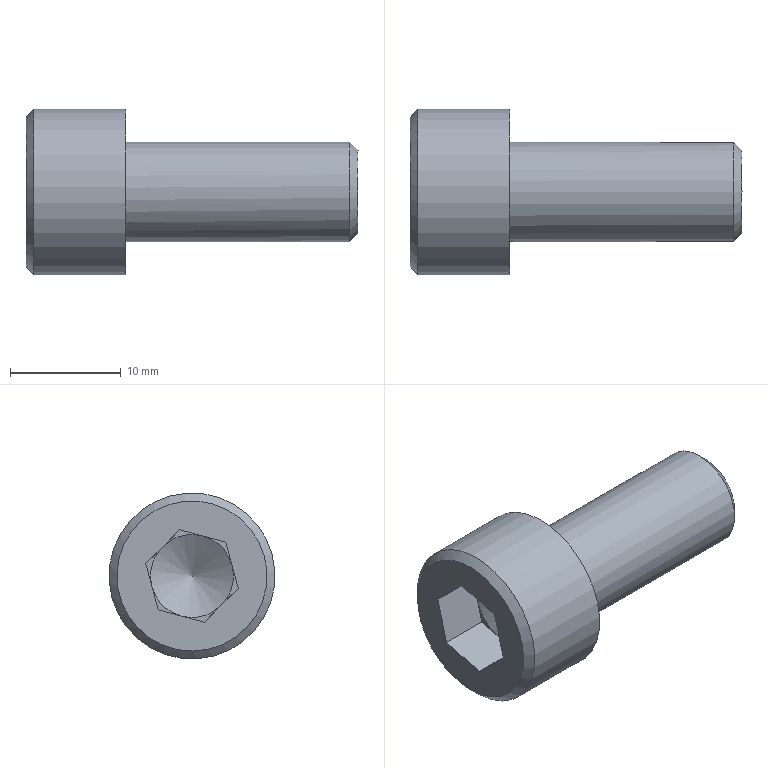Part | NX | features 切除-拉伸1 2 | 1 solid | 20 faces | box 30 x 15 x 15 mm | volume 2656 mm3 | plane 15 | cone 3 | cylinder 2 | commonest cylinder face diameters 9 x1 15 x1
STEP:
#1=CARTESIAN_POINT('',(-7.5,186.666,113.116));
#2=VERTEX_POINT('',#1);
#3=CARTESIAN_POINT('',(-7.5,186.666,109.366));
#4=DIRECTION('',(1.,0.,-0.000000019));
#5=DIRECTION('',(0.000000019,0.,1.));
#6=AXIS2_PLACEMENT_3D('',#3,#4,#5);
#7=CIRCLE('',#6,3.75);
#8=EDGE_CURVE('',#2,#2,#7,.T.);
#9=ORIENTED_EDGE('',*,*,#8,.T.);
#10=EDGE_LOOP('',(#9));
#11=FACE_BOUND('',#10,.T.);
#12=CARTESIAN_POINT('',(-7.5,239.166,109.366));
#13=DIRECTION('',(-1.,0.,0.000000019));
#14=DIRECTION('',(0.000000019,0.07719,0.997));
#15=AXIS2_PLACEMENT_3D('',#12,#13,#14);
#16=PLANE('',#15);
#17=ADVANCED_FACE('',(#11),#16,.F.);
#18=CARTESIAN_POINT('',(-8.25,186.666,113.866));
#19=VERTEX_POINT('',#18);
#20=CARTESIAN_POINT('',(-8.25,186.666,109.366));
#21=DIRECTION('',(1.,0.,-0.000000019));
#22=DIRECTION('',(0.000000019,0.,1.));
#23=AXIS2_PLACEMENT_3D('',#20,#21,#22);
#24=CIRCLE('',#23,4.5);
#25=EDGE_CURVE('',#19,#19,#24,.F.);
#26=ORIENTED_EDGE('',*,*,#25,.T.);
#27=EDGE_LOOP('',(#26));
#28=FACE_BOUND('',#27,.T.);
#29=CARTESIAN_POINT('',(-28.5,191.012,108.198));
#30=VERTEX_POINT('',#29);
#31=CARTESIAN_POINT('',(-28.5,186.666,109.366));
#32=DIRECTION('',(1.,0.,-0.000000019));
#33=DIRECTION('',(-0.000000005,0.9657,-0.2595));
#34=AXIS2_PLACEMENT_3D('',#31,#32,#33);
#35=CIRCLE('',#34,4.5);
#36=EDGE_CURVE('',#30,#30,#35,.F.);
#37=ORIENTED_EDGE('',*,*,#36,.F.);
#38=EDGE_LOOP('',(#37));
#39=FACE_BOUND('',#38,.T.);
#40=CARTESIAN_POINT('',(-40.125,186.666,109.366));
#41=DIRECTION('',(-1.,0.,0.000000019));
#42=DIRECTION('',(0.000000005,-0.9657,0.2595));
#43=AXIS2_PLACEMENT_3D('',#40,#41,#42);
#44=CYLINDRICAL_SURFACE('',#43,4.5);
#45=ADVANCED_FACE('',(#28,#39),#44,.T.);
#46=CARTESIAN_POINT('',(-33.,190.287,108.392));
#47=VERTEX_POINT('',#46);
#48=CARTESIAN_POINT('',(-33.,187.634,105.743));
#49=VERTEX_POINT('',#48);
#50=CARTESIAN_POINT('',(-33.,186.666,109.366));
#51=DIRECTION('',(1.,0.,-0.000000019));
#52=DIRECTION('',(-0.000000005,0.9657,-0.2595));
#53=AXIS2_PLACEMENT_3D('',#50,#51,#52);
#54=CIRCLE('',#53,3.75);
#55=EDGE_CURVE('',#47,#49,#54,.F.);
#56=ORIENTED_EDGE('',*,*,#55,.T.);
#57=CARTESIAN_POINT('',(-33.,184.012,106.716));
#58=VERTEX_POINT('',#57);
#59=CARTESIAN_POINT('',(-33.,186.666,109.366));
#60=DIRECTION('',(1.,0.,-0.000000019));
#61=DIRECTION('',(-0.000000005,0.9657,-0.2595));
#62=AXIS2_PLACEMENT_3D('',#59,#60,#61);
#63=CIRCLE('',#62,3.75);
#64=EDGE_CURVE('',#49,#58,#63,.F.);
#65=ORIENTED_EDGE('',*,*,#64,.T.);
#66=CARTESIAN_POINT('',(-33.,183.044,110.339));
#67=VERTEX_POINT('',#66);
#68=CARTESIAN_POINT('',(-33.,186.666,109.366));
#69=DIRECTION('',(1.,0.,-0.000000019));
#70=DIRECTION('',(-0.000000005,0.9657,-0.2595));
#71=AXIS2_PLACEMENT_3D('',#68,#69,#70);
#72=CIRCLE('',#71,3.75);
#73=EDGE_CURVE('',#58,#67,#72,.F.);
#74=ORIENTED_EDGE('',*,*,#73,.T.);
#75=CARTESIAN_POINT('',(-33.,185.698,112.989));
#76=VERTEX_POINT('',#75);
#77=CARTESIAN_POINT('',(-33.,186.666,109.366));
#78=DIRECTION('',(1.,0.,-0.000000019));
#79=DIRECTION('',(-0.000000005,0.9657,-0.2595));
#80=AXIS2_PLACEMENT_3D('',#77,#78,#79);
#81=CIRCLE('',#80,3.75);
#82=EDGE_CURVE('',#67,#76,#81,.F.);
#83=ORIENTED_EDGE('',*,*,#82,.T.);
#84=CARTESIAN_POINT('',(-33.,189.319,112.015));
#85=VERTEX_POINT('',#84);
#86=CARTESIAN_POINT('',(-33.,186.666,109.366));
#87=DIRECTION('',(1.,0.,-0.000000019));
#88=DIRECTION('',(-0.000000005,0.9657,-0.2595));
#89=AXIS2_PLACEMENT_3D('',#86,#87,#88);
#90=CIRCLE('',#89,3.75);
#91=EDGE_CURVE('',#76,#85,#90,.F.);
#92=ORIENTED_EDGE('',*,*,#91,.T.);
#93=CARTESIAN_POINT('',(-33.,186.666,109.366));
#94=DIRECTION('',(1.,0.,-0.000000019));
#95=DIRECTION('',(-0.000000005,0.9657,-0.2595));
#96=AXIS2_PLACEMENT_3D('',#93,#94,#95);
#97=CIRCLE('',#96,3.75);
#98=EDGE_CURVE('',#85,#47,#97,.F.);
#99=ORIENTED_EDGE('',*,*,#98,.T.);
#100=EDGE_LOOP('',(#56,#65,#74,#83,#92,#99));
#101=FACE_BOUND('',#100,.T.);
#102=CARTESIAN_POINT('',(-30.835,186.666,109.366));
#103=VERTEX_POINT('',#102);
#104=VERTEX_LOOP('',#103);
#105=FACE_BOUND('',#104,.T.);
#106=CARTESIAN_POINT('',(-33.,186.666,109.366));
#107=DIRECTION('',(-1.,0.,0.000000019));
#108=DIRECTION('',(0.000000005,-0.9657,0.2595));
#109=AXIS2_PLACEMENT_3D('',#106,#107,#108);
#110=CONICAL_SURFACE('',#109,3.75,1.047);
#111=ADVANCED_FACE('',(#101,#105),#110,.F.);
#112=CARTESIAN_POINT('',(-36.78,179.423,111.312));
#113=VERTEX_POINT('',#112);
#114=CARTESIAN_POINT('',(-36.78,186.666,109.366));
#115=DIRECTION('',(-1.,0.,0.000000019));
#116=DIRECTION('',(0.000000005,-0.9657,0.2595));
#117=AXIS2_PLACEMENT_3D('',#114,#115,#116);
#118=CIRCLE('',#117,7.5);
#119=EDGE_CURVE('',#113,#113,#118,.F.);
#120=ORIENTED_EDGE('',*,*,#119,.F.);
#121=EDGE_LOOP('',(#120));
#122=FACE_BOUND('',#121,.T.);
#123=CARTESIAN_POINT('',(-37.5,180.118,111.125));
#124=VERTEX_POINT('',#123);
#125=CARTESIAN_POINT('',(-37.5,186.666,109.366));
#126=DIRECTION('',(1.,0.,-0.000000019));
#127=DIRECTION('',(0.000000005,-0.9657,0.2595));
#128=AXIS2_PLACEMENT_3D('',#125,#126,#127);
#129=CIRCLE('',#128,6.78);
#130=EDGE_CURVE('',#124,#124,#129,.F.);
#131=ORIENTED_EDGE('',*,*,#130,.F.);
#132=EDGE_LOOP('',(#131));
#133=FACE_BOUND('',#132,.T.);
#134=CARTESIAN_POINT('',(-37.5,186.666,109.366));
#135=DIRECTION('',(1.,0.,-0.000000019));
#136=DIRECTION('',(-0.000000005,0.9657,-0.2595));
#137=AXIS2_PLACEMENT_3D('',#134,#135,#136);
#138=CONICAL_SURFACE('',#137,6.78,0.7854);
#139=ADVANCED_FACE('',(#122,#133),#138,.T.);
#140=ORIENTED_EDGE('',*,*,#119,.T.);
#141=EDGE_LOOP('',(#140));
#142=FACE_BOUND('',#141,.T.);
#143=CARTESIAN_POINT('',(-28.5,193.909,107.419));
#144=VERTEX_POINT('',#143);
#145=CARTESIAN_POINT('',(-28.5,186.666,109.366));
#146=DIRECTION('',(1.,0.,-0.000000019));
#147=DIRECTION('',(-0.000000005,0.9657,-0.2595));
#148=AXIS2_PLACEMENT_3D('',#145,#146,#147);
#149=CIRCLE('',#148,7.5);
#150=EDGE_CURVE('',#144,#144,#149,.F.);
#151=ORIENTED_EDGE('',*,*,#150,.T.);
#152=EDGE_LOOP('',(#151));
#153=FACE_BOUND('',#152,.T.);
#154=CARTESIAN_POINT('',(-40.125,186.666,109.366));
#155=DIRECTION('',(-1.,0.,0.000000019));
#156=DIRECTION('',(0.000000005,-0.9657,0.2595));
#157=AXIS2_PLACEMENT_3D('',#154,#155,#156);
#158=CYLINDRICAL_SURFACE('',#157,7.5);
#159=ADVANCED_FACE('',(#142,#153),#158,.T.);
#160=ORIENTED_EDGE('',*,*,#130,.T.);
#161=EDGE_LOOP('',(#160));
#162=FACE_BOUND('',#161,.T.);
#163=CARTESIAN_POINT('',(-37.5,187.79,113.547));
#164=VERTEX_POINT('',#163);
#165=CARTESIAN_POINT('',(-37.5,183.606,112.43));
#166=VERTEX_POINT('',#165);
#167=CARTESIAN_POINT('',(-37.5,182.56,112.151));
#168=DIRECTION('',(0.000000005,0.9661,0.2581));
#169=VECTOR('',#168,1000.);
#170=LINE('',#167,#169);
#171=EDGE_CURVE('',#164,#166,#170,.F.);
#172=ORIENTED_EDGE('',*,*,#171,.T.);
#173=CARTESIAN_POINT('',(-37.5,182.482,108.248));
#174=VERTEX_POINT('',#173);
#175=CARTESIAN_POINT('',(-37.5,183.044,110.339));
#176=DIRECTION('',(0.000000018,0.2595,0.9657));
#177=VECTOR('',#176,1000.);
#178=LINE('',#175,#177);
#179=EDGE_CURVE('',#166,#174,#178,.F.);
#180=ORIENTED_EDGE('',*,*,#179,.T.);
#181=CARTESIAN_POINT('',(-37.5,185.542,105.184));
#182=VERTEX_POINT('',#181);
#183=CARTESIAN_POINT('',(-37.5,181.717,109.014));
#184=DIRECTION('',(0.000000013,-0.7066,0.7076));
#185=VECTOR('',#184,1000.);
#186=LINE('',#183,#185);
#187=EDGE_CURVE('',#174,#182,#186,.F.);
#188=ORIENTED_EDGE('',*,*,#187,.T.);
#189=CARTESIAN_POINT('',(-37.5,189.725,106.302));
#190=VERTEX_POINT('',#189);
#191=CARTESIAN_POINT('',(-37.5,184.496,104.905));
#192=DIRECTION('',(-0.000000005,-0.9661,-0.2581));
#193=VECTOR('',#192,1000.);
#194=LINE('',#191,#193);
#195=EDGE_CURVE('',#182,#190,#194,.F.);
#196=ORIENTED_EDGE('',*,*,#195,.T.);
#197=CARTESIAN_POINT('',(-37.5,190.849,110.483));
#198=VERTEX_POINT('',#197);
#199=CARTESIAN_POINT('',(-37.5,190.287,108.392));
#200=DIRECTION('',(-0.000000018,-0.2595,-0.9657));
#201=VECTOR('',#200,1000.);
#202=LINE('',#199,#201);
#203=EDGE_CURVE('',#190,#198,#202,.F.);
#204=ORIENTED_EDGE('',*,*,#203,.T.);
#205=CARTESIAN_POINT('',(-37.5,187.025,114.314));
#206=DIRECTION('',(-0.000000013,0.7066,-0.7076));
#207=VECTOR('',#206,1000.);
#208=LINE('',#205,#207);
#209=EDGE_CURVE('',#198,#164,#208,.F.);
#210=ORIENTED_EDGE('',*,*,#209,.T.);
#211=EDGE_LOOP('',(#172,#180,#188,#196,#204,#210));
#212=FACE_BOUND('',#211,.T.);
#213=CARTESIAN_POINT('',(-37.5,183.044,110.339));
#214=DIRECTION('',(1.,0.,-0.000000019));
#215=DIRECTION('',(-0.000000005,0.9657,-0.2595));
#216=AXIS2_PLACEMENT_3D('',#213,#214,#215);
#217=PLANE('',#216);
#218=ADVANCED_FACE('',(#162,#212),#217,.F.);
#219=ORIENTED_EDGE('',*,*,#150,.F.);
#220=EDGE_LOOP('',(#219));
#221=FACE_BOUND('',#220,.T.);
#222=ORIENTED_EDGE('',*,*,#36,.T.);
#223=EDGE_LOOP('',(#222));
#224=FACE_BOUND('',#223,.T.);
#225=CARTESIAN_POINT('',(-28.5,179.423,111.312));
#226=DIRECTION('',(-1.,0.,0.000000019));
#227=DIRECTION('',(0.000000005,-0.9657,0.2595));
#228=AXIS2_PLACEMENT_3D('',#225,#226,#227);
#229=PLANE('',#228);
#230=ADVANCED_FACE('',(#221,#224),#229,.F.);
#231=ORIENTED_EDGE('',*,*,#98,.F.);
#232=CARTESIAN_POINT('',(-33.,190.849,110.483));
#233=VERTEX_POINT('',#232);
#234=CARTESIAN_POINT('',(-33.,190.849,110.483));
#235=DIRECTION('',(0.000000013,-0.7066,0.7076));
#236=VECTOR('',#235,1000.);
#237=LINE('',#234,#236);
#238=EDGE_CURVE('',#85,#233,#237,.F.);
#239=ORIENTED_EDGE('',*,*,#238,.T.);
#240=CARTESIAN_POINT('',(-33.,189.725,106.302));
#241=DIRECTION('',(0.000000018,0.2595,0.9657));
#242=VECTOR('',#241,1000.);
#243=LINE('',#240,#242);
#244=EDGE_CURVE('',#233,#47,#243,.F.);
#245=ORIENTED_EDGE('',*,*,#244,.T.);
#246=EDGE_LOOP('',(#231,#239,#245));
#247=FACE_BOUND('',#246,.T.);
#248=CARTESIAN_POINT('',(-33.,186.666,109.366));
#249=DIRECTION('',(-1.,0.,0.000000019));
#250=DIRECTION('',(-0.000000018,-0.2595,-0.9657));
#251=AXIS2_PLACEMENT_3D('',#248,#249,#250);
#252=PLANE('',#251);
#253=ADVANCED_FACE('',(#247),#252,.T.);
#254=ORIENTED_EDGE('',*,*,#55,.F.);
#255=CARTESIAN_POINT('',(-33.,189.725,106.302));
#256=VERTEX_POINT('',#255);
#257=CARTESIAN_POINT('',(-33.,189.725,106.302));
#258=DIRECTION('',(0.000000018,0.2595,0.9657));
#259=VECTOR('',#258,1000.);
#260=LINE('',#257,#259);
#261=EDGE_CURVE('',#47,#256,#260,.F.);
#262=ORIENTED_EDGE('',*,*,#261,.T.);
#263=CARTESIAN_POINT('',(-33.,185.542,105.184));
#264=DIRECTION('',(0.000000005,0.9661,0.2581));
#265=VECTOR('',#264,1000.);
#266=LINE('',#263,#265);
#267=EDGE_CURVE('',#256,#49,#266,.F.);
#268=ORIENTED_EDGE('',*,*,#267,.T.);
#269=EDGE_LOOP('',(#254,#262,#268));
#270=FACE_BOUND('',#269,.T.);
#271=CARTESIAN_POINT('',(-33.,186.666,109.366));
#272=DIRECTION('',(-1.,0.,0.000000019));
#273=DIRECTION('',(-0.000000018,-0.2595,-0.9657));
#274=AXIS2_PLACEMENT_3D('',#271,#272,#273);
#275=PLANE('',#274);
#276=ADVANCED_FACE('',(#270),#275,.T.);
#277=ORIENTED_EDGE('',*,*,#64,.F.);
#278=CARTESIAN_POINT('',(-33.,185.542,105.184));
#279=VERTEX_POINT('',#278);
#280=CARTESIAN_POINT('',(-33.,185.542,105.184));
#281=DIRECTION('',(0.000000005,0.9661,0.2581));
#282=VECTOR('',#281,1000.);
#283=LINE('',#280,#282);
#284=EDGE_CURVE('',#49,#279,#283,.F.);
#285=ORIENTED_EDGE('',*,*,#284,.T.);
#286=CARTESIAN_POINT('',(-33.,182.482,108.248));
#287=DIRECTION('',(-0.000000013,0.7066,-0.7076));
#288=VECTOR('',#287,1000.);
#289=LINE('',#286,#288);
#290=EDGE_CURVE('',#279,#58,#289,.F.);
#291=ORIENTED_EDGE('',*,*,#290,.T.);
#292=EDGE_LOOP('',(#277,#285,#291));
#293=FACE_BOUND('',#292,.T.);
#294=CARTESIAN_POINT('',(-33.,186.666,109.366));
#295=DIRECTION('',(-1.,0.,0.000000019));
#296=DIRECTION('',(-0.000000018,-0.2595,-0.9657));
#297=AXIS2_PLACEMENT_3D('',#294,#295,#296);
#298=PLANE('',#297);
#299=ADVANCED_FACE('',(#293),#298,.T.);
#300=ORIENTED_EDGE('',*,*,#73,.F.);
#301=CARTESIAN_POINT('',(-33.,182.482,108.248));
#302=VERTEX_POINT('',#301);
#303=CARTESIAN_POINT('',(-33.,182.482,108.248));
#304=DIRECTION('',(-0.000000013,0.7066,-0.7076));
#305=VECTOR('',#304,1000.);
#306=LINE('',#303,#305);
#307=EDGE_CURVE('',#58,#302,#306,.F.);
#308=ORIENTED_EDGE('',*,*,#307,.T.);
#309=CARTESIAN_POINT('',(-33.,183.606,112.43));
#310=DIRECTION('',(-0.000000018,-0.2595,-0.9657));
#311=VECTOR('',#310,1000.);
#312=LINE('',#309,#311);
#313=EDGE_CURVE('',#302,#67,#312,.F.);
#314=ORIENTED_EDGE('',*,*,#313,.T.);
#315=EDGE_LOOP('',(#300,#308,#314));
#316=FACE_BOUND('',#315,.T.);
#317=CARTESIAN_POINT('',(-33.,186.666,109.366));
#318=DIRECTION('',(-1.,0.,0.000000019));
#319=DIRECTION('',(-0.000000018,-0.2595,-0.9657));
#320=AXIS2_PLACEMENT_3D('',#317,#318,#319);
#321=PLANE('',#320);
#322=ADVANCED_FACE('',(#316),#321,.T.);
#323=ORIENTED_EDGE('',*,*,#82,.F.);
#324=CARTESIAN_POINT('',(-33.,183.606,112.43));
#325=VERTEX_POINT('',#324);
#326=CARTESIAN_POINT('',(-33.,183.606,112.43));
#327=DIRECTION('',(-0.000000018,-0.2595,-0.9657));
#328=VECTOR('',#327,1000.);
#329=LINE('',#326,#328);
#330=EDGE_CURVE('',#67,#325,#329,.F.);
#331=ORIENTED_EDGE('',*,*,#330,.T.);
#332=CARTESIAN_POINT('',(-33.,187.79,113.547));
#333=DIRECTION('',(-0.000000005,-0.9661,-0.2581));
#334=VECTOR('',#333,1000.);
#335=LINE('',#332,#334);
#336=EDGE_CURVE('',#325,#76,#335,.F.);
#337=ORIENTED_EDGE('',*,*,#336,.T.);
#338=EDGE_LOOP('',(#323,#331,#337));
#339=FACE_BOUND('',#338,.T.);
#340=CARTESIAN_POINT('',(-33.,186.666,109.366));
#341=DIRECTION('',(-1.,0.,0.000000019));
#342=DIRECTION('',(-0.000000018,-0.2595,-0.9657));
#343=AXIS2_PLACEMENT_3D('',#340,#341,#342);
#344=PLANE('',#343);
#345=ADVANCED_FACE('',(#339),#344,.T.);
#346=ORIENTED_EDGE('',*,*,#91,.F.);
#347=CARTESIAN_POINT('',(-33.,187.79,113.547));
#348=VERTEX_POINT('',#347);
#349=CARTESIAN_POINT('',(-33.,187.79,113.547));
#350=DIRECTION('',(-0.000000005,-0.9661,-0.2581));
#351=VECTOR('',#350,1000.);
#352=LINE('',#349,#351);
#353=EDGE_CURVE('',#76,#348,#352,.F.);
#354=ORIENTED_EDGE('',*,*,#353,.T.);
#355=CARTESIAN_POINT('',(-33.,190.849,110.483));
#356=DIRECTION('',(0.000000013,-0.7066,0.7076));
#357=VECTOR('',#356,1000.);
#358=LINE('',#355,#357);
#359=EDGE_CURVE('',#348,#85,#358,.F.);
#360=ORIENTED_EDGE('',*,*,#359,.T.);
#361=EDGE_LOOP('',(#346,#354,#360));
#362=FACE_BOUND('',#361,.T.);
#363=CARTESIAN_POINT('',(-33.,186.666,109.366));
#364=DIRECTION('',(-1.,0.,0.000000019));
#365=DIRECTION('',(-0.000000018,-0.2595,-0.9657));
#366=AXIS2_PLACEMENT_3D('',#363,#364,#365);
#367=PLANE('',#366);
#368=ADVANCED_FACE('',(#362),#367,.T.);
#369=ORIENTED_EDGE('',*,*,#209,.F.);
#370=CARTESIAN_POINT('',(-33.,190.849,110.483));
#371=DIRECTION('',(-1.,0.,0.000000019));
#372=VECTOR('',#371,1000.);
#373=LINE('',#370,#372);
#374=EDGE_CURVE('',#198,#233,#373,.F.);
#375=ORIENTED_EDGE('',*,*,#374,.T.);
#376=ORIENTED_EDGE('',*,*,#238,.F.);
#377=ORIENTED_EDGE('',*,*,#359,.F.);
#378=CARTESIAN_POINT('',(-33.,187.79,113.547));
#379=DIRECTION('',(-1.,0.,0.000000019));
#380=VECTOR('',#379,1000.);
#381=LINE('',#378,#380);
#382=EDGE_CURVE('',#164,#348,#381,.F.);
#383=ORIENTED_EDGE('',*,*,#382,.F.);
#384=EDGE_LOOP('',(#369,#375,#376,#377,#383));
#385=FACE_BOUND('',#384,.T.);
#386=CARTESIAN_POINT('',(-33.,190.849,110.483));
#387=DIRECTION('',(0.000000013,0.7076,0.7066));
#388=DIRECTION('',(0.000000013,-0.7066,0.7076));
#389=AXIS2_PLACEMENT_3D('',#386,#387,#388);
#390=PLANE('',#389);
#391=ADVANCED_FACE('',(#385),#390,.F.);
#392=ORIENTED_EDGE('',*,*,#203,.F.);
#393=CARTESIAN_POINT('',(-33.,189.725,106.302));
#394=DIRECTION('',(-1.,0.,0.000000019));
#395=VECTOR('',#394,1000.);
#396=LINE('',#393,#395);
#397=EDGE_CURVE('',#190,#256,#396,.F.);
#398=ORIENTED_EDGE('',*,*,#397,.T.);
#399=ORIENTED_EDGE('',*,*,#261,.F.);
#400=ORIENTED_EDGE('',*,*,#244,.F.);
#401=ORIENTED_EDGE('',*,*,#374,.F.);
#402=EDGE_LOOP('',(#392,#398,#399,#400,#401));
#403=FACE_BOUND('',#402,.T.);
#404=CARTESIAN_POINT('',(-33.,189.725,106.302));
#405=DIRECTION('',(-0.000000005,0.9657,-0.2595));
#406=DIRECTION('',(-1.,0.,0.000000019));
#407=AXIS2_PLACEMENT_3D('',#404,#405,#406);
#408=PLANE('',#407);
#409=ADVANCED_FACE('',(#403),#408,.F.);
#410=ORIENTED_EDGE('',*,*,#195,.F.);
#411=CARTESIAN_POINT('',(-33.,185.542,105.184));
#412=DIRECTION('',(-1.,0.,0.000000019));
#413=VECTOR('',#412,1000.);
#414=LINE('',#411,#413);
#415=EDGE_CURVE('',#182,#279,#414,.F.);
#416=ORIENTED_EDGE('',*,*,#415,.T.);
#417=ORIENTED_EDGE('',*,*,#284,.F.);
#418=ORIENTED_EDGE('',*,*,#267,.F.);
#419=ORIENTED_EDGE('',*,*,#397,.F.);
#420=EDGE_LOOP('',(#410,#416,#417,#418,#419));
#421=FACE_BOUND('',#420,.T.);
#422=CARTESIAN_POINT('',(-33.,185.542,105.184));
#423=DIRECTION('',(-0.000000018,0.2581,-0.9661));
#424=DIRECTION('',(0.000000005,0.9661,0.2581));
#425=AXIS2_PLACEMENT_3D('',#422,#423,#424);
#426=PLANE('',#425);
#427=ADVANCED_FACE('',(#421),#426,.F.);
#428=ORIENTED_EDGE('',*,*,#187,.F.);
#429=CARTESIAN_POINT('',(-33.,182.482,108.248));
#430=DIRECTION('',(-1.,0.,0.000000019));
#431=VECTOR('',#430,1000.);
#432=LINE('',#429,#431);
#433=EDGE_CURVE('',#174,#302,#432,.F.);
#434=ORIENTED_EDGE('',*,*,#433,.T.);
#435=ORIENTED_EDGE('',*,*,#307,.F.);
#436=ORIENTED_EDGE('',*,*,#290,.F.);
#437=ORIENTED_EDGE('',*,*,#415,.F.);
#438=EDGE_LOOP('',(#428,#434,#435,#436,#437));
#439=FACE_BOUND('',#438,.T.);
#440=CARTESIAN_POINT('',(-33.,182.482,108.248));
#441=DIRECTION('',(-0.000000013,-0.7076,-0.7066));
#442=DIRECTION('',(-0.000000013,0.7066,-0.7076));
#443=AXIS2_PLACEMENT_3D('',#440,#441,#442);
#444=PLANE('',#443);
#445=ADVANCED_FACE('',(#439),#444,.F.);
#446=ORIENTED_EDGE('',*,*,#179,.F.);
#447=CARTESIAN_POINT('',(-33.,183.606,112.43));
#448=DIRECTION('',(-1.,0.,0.000000019));
#449=VECTOR('',#448,1000.);
#450=LINE('',#447,#449);
#451=EDGE_CURVE('',#166,#325,#450,.F.);
#452=ORIENTED_EDGE('',*,*,#451,.T.);
#453=ORIENTED_EDGE('',*,*,#330,.F.);
#454=ORIENTED_EDGE('',*,*,#313,.F.);
#455=ORIENTED_EDGE('',*,*,#433,.F.);
#456=EDGE_LOOP('',(#446,#452,#453,#454,#455));
#457=FACE_BOUND('',#456,.T.);
#458=CARTESIAN_POINT('',(-33.,183.606,112.43));
#459=DIRECTION('',(0.000000005,-0.9657,0.2595));
#460=DIRECTION('',(1.,0.,-0.000000019));
#461=AXIS2_PLACEMENT_3D('',#458,#459,#460);
#462=PLANE('',#461);
#463=ADVANCED_FACE('',(#457),#462,.F.);
#464=ORIENTED_EDGE('',*,*,#171,.F.);
#465=ORIENTED_EDGE('',*,*,#382,.T.);
#466=ORIENTED_EDGE('',*,*,#353,.F.);
#467=ORIENTED_EDGE('',*,*,#336,.F.);
#468=ORIENTED_EDGE('',*,*,#451,.F.);
#469=EDGE_LOOP('',(#464,#465,#466,#467,#468));
#470=FACE_BOUND('',#469,.T.);
#471=CARTESIAN_POINT('',(-33.,187.79,113.547));
#472=DIRECTION('',(0.000000018,-0.2581,0.9661));
#473=DIRECTION('',(-0.000000005,-0.9661,-0.2581));
#474=AXIS2_PLACEMENT_3D('',#471,#472,#473);
#475=PLANE('',#474);
#476=ADVANCED_FACE('',(#470),#475,.F.);
#477=ORIENTED_EDGE('',*,*,#8,.F.);
#478=EDGE_LOOP('',(#477));
#479=FACE_BOUND('',#478,.T.);
#480=ORIENTED_EDGE('',*,*,#25,.F.);
#481=EDGE_LOOP('',(#480));
#482=FACE_BOUND('',#481,.T.);
#483=CARTESIAN_POINT('',(-8.25,186.666,109.366));
#484=DIRECTION('',(-1.,0.,0.000000019));
#485=DIRECTION('',(0.000000019,0.,1.));
#486=AXIS2_PLACEMENT_3D('',#483,#484,#485);
#487=CONICAL_SURFACE('',#486,4.5,0.7854);
#488=ADVANCED_FACE('',(#479,#482),#487,.T.);
#489=CLOSED_SHELL('',(#17,#45,#111,#139,#159,#218,#230,#253,#276,#299,#322,#345,#368,#391,#409,#427,#445,#463,#476,#488));
#490=MANIFOLD_SOLID_BREP('',#489);
#491=(LENGTH_UNIT()NAMED_UNIT(*)SI_UNIT(.MILLI.,.METRE.));
#492=UNCERTAINTY_MEASURE_WITH_UNIT(LENGTH_MEASURE(0.00001),#491,'','');
#493=(NAMED_UNIT(*)PLANE_ANGLE_UNIT()SI_UNIT($,.RADIAN.));
#494=(NAMED_UNIT(*)SI_UNIT($,.STERADIAN.)SOLID_ANGLE_UNIT());
#495=(GEOMETRIC_REPRESENTATION_CONTEXT(3)GLOBAL_UNCERTAINTY_ASSIGNED_CONTEXT((#492))GLOBAL_UNIT_ASSIGNED_CONTEXT((#491,#493,#494))REPRESENTATION_CONTEXT('',''));
#496=ADVANCED_BREP_SHAPE_REPRESENTATION('',(#490),#495);